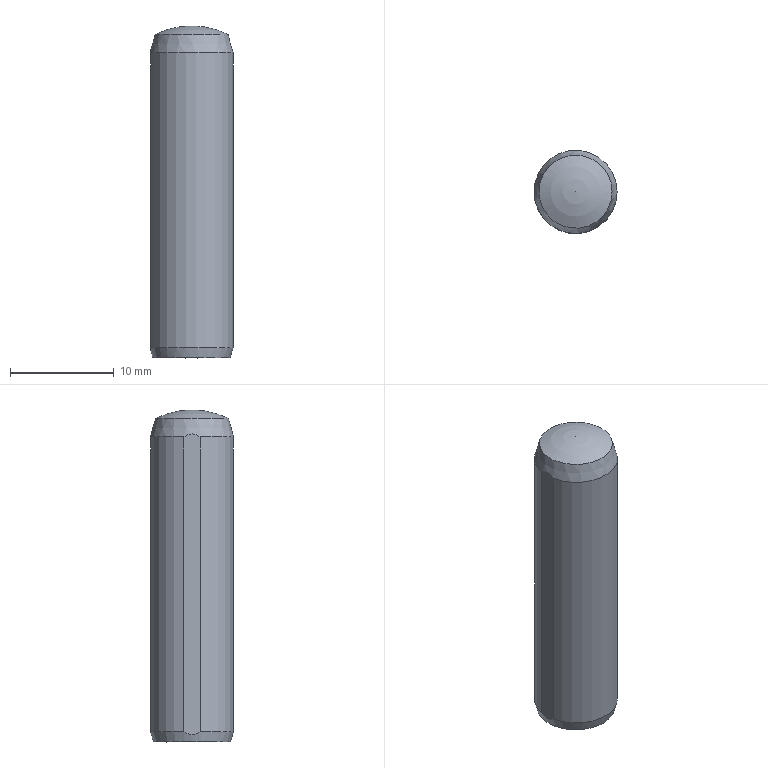Part | STEP file | 1_18 | 1 solid | 12 faces | box 7.92 x 8 x 32 mm | volume 1366 mm3 | cone 5 | cylinder 3 | plane 3 | sphere 1 | commonest cylinder face diameters 4.134 x2 8 x1
STEP:
#1=CARTESIAN_POINT('',(0.,0.,0.));
#2=DIRECTION('',(0.,0.,1.));
#3=DIRECTION('',(1.,0.,0.));
#4=AXIS2_PLACEMENT_3D('',#1,#2,#3);
#5=CARTESIAN_POINT('',(-3.92,-0.796,29.4));
#6=VERTEX_POINT('',#5);
#7=CARTESIAN_POINT('',(-3.92,0.796,29.4));
#8=VERTEX_POINT('',#7);
#9=CARTESIAN_POINT('',(0.,0.,29.4));
#10=DIRECTION('',(0.,0.,1.));
#11=DIRECTION('',(1.,0.,0.));
#12=AXIS2_PLACEMENT_3D('',#9,#10,#11);
#13=CIRCLE('',#12,4.);
#14=CARTESIAN_POINT('',(0.,0.,15.2));
#15=DIRECTION('',(0.,0.,1.));
#16=DIRECTION('',(0.,1.,0.));
#17=AXIS2_PLACEMENT_3D('',#14,#15,#16);
#18=CYLINDRICAL_SURFACE('',#17,4.);
#19=CARTESIAN_POINT('',(-1.571,14.2));
#20=DIRECTION('',(1.,0.));
#21=VECTOR('',#20,1.);
#22=LINE('',#19,#21);
#23=(GEOMETRIC_REPRESENTATION_CONTEXT(2)PARAMETRIC_REPRESENTATION_CONTEXT()REPRESENTATION_CONTEXT('',''));
#24=DEFINITIONAL_REPRESENTATION('',(#22),#23);
#25=PCURVE('',#18,#24);
#26=CARTESIAN_POINT('',(0.,0.,30.291));
#27=DIRECTION('',(0.,0.,-1.));
#28=DIRECTION('',(0.,-1.,0.));
#29=AXIS2_PLACEMENT_3D('',#26,#27,#28);
#30=CONICAL_SURFACE('',#29,3.761,0.2618);
#31=CARTESIAN_POINT('',(10.996,0.8914));
#32=DIRECTION('',(-1.,0.));
#33=VECTOR('',#32,1.);
#34=LINE('',#31,#33);
#35=(GEOMETRIC_REPRESENTATION_CONTEXT(2)PARAMETRIC_REPRESENTATION_CONTEXT()REPRESENTATION_CONTEXT('',''));
#36=DEFINITIONAL_REPRESENTATION('',(#34),#35);
#37=PCURVE('',#30,#36);
#38=SURFACE_CURVE('',#13,(#25,#37),.PCURVE_S1.);
#39=EDGE_CURVE('',#6,#8,#38,.T.);
#40=ORIENTED_EDGE('',*,*,#39,.F.);
#41=CARTESIAN_POINT('',(-3.92,-0.796,1.));
#42=VERTEX_POINT('',#41);
#43=CARTESIAN_POINT('',(-3.92,-0.796,1.));
#44=DIRECTION('',(0.,0.,1.));
#45=VECTOR('',#44,1.);
#46=LINE('',#43,#45);
#47=CARTESIAN_POINT('',(1.771,-14.2));
#48=DIRECTION('',(0.,1.));
#49=VECTOR('',#48,1.);
#50=LINE('',#47,#49);
#51=(GEOMETRIC_REPRESENTATION_CONTEXT(2)PARAMETRIC_REPRESENTATION_CONTEXT()REPRESENTATION_CONTEXT('',''));
#52=DEFINITIONAL_REPRESENTATION('',(#50),#51);
#53=PCURVE('',#18,#52);
#54=CARTESIAN_POINT('',(-3.92,0.,15.9));
#55=DIRECTION('',(-1.,0.,0.));
#56=DIRECTION('',(0.,0.,1.));
#57=AXIS2_PLACEMENT_3D('',#54,#55,#56);
#58=PLANE('',#57);
#59=CARTESIAN_POINT('',(-14.9,-0.796));
#60=DIRECTION('',(1.,0.));
#61=VECTOR('',#60,1.);
#62=LINE('',#59,#61);
#63=(GEOMETRIC_REPRESENTATION_CONTEXT(2)PARAMETRIC_REPRESENTATION_CONTEXT()REPRESENTATION_CONTEXT('',''));
#64=DEFINITIONAL_REPRESENTATION('',(#62),#63);
#65=PCURVE('',#58,#64);
#66=SURFACE_CURVE('',#46,(#53,#65),.PCURVE_S1.);
#67=EDGE_CURVE('',#42,#6,#66,.T.);
#68=ORIENTED_EDGE('',*,*,#67,.F.);
#69=CARTESIAN_POINT('',(-3.92,0.796,1.));
#70=VERTEX_POINT('',#69);
#71=CARTESIAN_POINT('',(0.,0.,1.));
#72=DIRECTION('',(0.,0.,1.));
#73=DIRECTION('',(1.,0.,0.));
#74=AXIS2_PLACEMENT_3D('',#71,#72,#73);
#75=CIRCLE('',#74,4.);
#76=CARTESIAN_POINT('',(-1.571,-14.2));
#77=DIRECTION('',(1.,0.));
#78=VECTOR('',#77,1.);
#79=LINE('',#76,#78);
#80=(GEOMETRIC_REPRESENTATION_CONTEXT(2)PARAMETRIC_REPRESENTATION_CONTEXT()REPRESENTATION_CONTEXT('',''));
#81=DEFINITIONAL_REPRESENTATION('',(#79),#80);
#82=PCURVE('',#18,#81);
#83=CARTESIAN_POINT('',(0.,0.,0.5));
#84=DIRECTION('',(0.,0.,1.));
#85=DIRECTION('',(0.,1.,0.));
#86=AXIS2_PLACEMENT_3D('',#83,#84,#85);
#87=CONICAL_SURFACE('',#86,3.866,0.2618);
#88=CARTESIAN_POINT('',(-1.571,0.5));
#89=DIRECTION('',(1.,0.));
#90=VECTOR('',#89,1.);
#91=LINE('',#88,#90);
#92=(GEOMETRIC_REPRESENTATION_CONTEXT(2)PARAMETRIC_REPRESENTATION_CONTEXT()REPRESENTATION_CONTEXT('',''));
#93=DEFINITIONAL_REPRESENTATION('',(#91),#92);
#94=PCURVE('',#87,#93);
#95=SURFACE_CURVE('',#75,(#82,#94),.PCURVE_S1.);
#96=EDGE_CURVE('',#42,#70,#95,.T.);
#97=ORIENTED_EDGE('',*,*,#96,.T.);
#98=CARTESIAN_POINT('',(-3.92,0.796,1.));
#99=DIRECTION('',(0.,0.,1.));
#100=VECTOR('',#99,1.);
#101=LINE('',#98,#100);
#102=CARTESIAN_POINT('',(7.654,-14.2));
#103=DIRECTION('',(0.,1.));
#104=VECTOR('',#103,1.);
#105=LINE('',#102,#104);
#106=(GEOMETRIC_REPRESENTATION_CONTEXT(2)PARAMETRIC_REPRESENTATION_CONTEXT()REPRESENTATION_CONTEXT('',''));
#107=DEFINITIONAL_REPRESENTATION('',(#105),#106);
#108=PCURVE('',#18,#107);
#109=CARTESIAN_POINT('',(-14.9,0.796));
#110=DIRECTION('',(1.,0.));
#111=VECTOR('',#110,1.);
#112=LINE('',#109,#111);
#113=(GEOMETRIC_REPRESENTATION_CONTEXT(2)PARAMETRIC_REPRESENTATION_CONTEXT()REPRESENTATION_CONTEXT('',''));
#114=DEFINITIONAL_REPRESENTATION('',(#112),#113);
#115=PCURVE('',#58,#114);
#116=SURFACE_CURVE('',#101,(#108,#115),.PCURVE_S1.);
#117=EDGE_CURVE('',#70,#8,#116,.T.);
#118=ORIENTED_EDGE('',*,*,#117,.T.);
#119=EDGE_LOOP('',(#40,#68,#97,#118));
#120=FACE_BOUND('',#119,.T.);
#121=ADVANCED_FACE('',(#120),#18,.T.);
#122=CARTESIAN_POINT('',(-3.522,0.,31.183));
#123=VERTEX_POINT('',#122);
#124=CARTESIAN_POINT('',(3.522,0.,31.183));
#125=VERTEX_POINT('',#124);
#126=CARTESIAN_POINT('',(0.,0.,31.183));
#127=DIRECTION('',(0.,0.,-1.));
#128=DIRECTION('',(1.,0.,0.));
#129=AXIS2_PLACEMENT_3D('',#126,#127,#128);
#130=CIRCLE('',#129,3.522);
#131=CARTESIAN_POINT('',(-1.571,-0.8914));
#132=DIRECTION('',(1.,0.));
#133=VECTOR('',#132,1.);
#134=LINE('',#131,#133);
#135=(GEOMETRIC_REPRESENTATION_CONTEXT(2)PARAMETRIC_REPRESENTATION_CONTEXT()REPRESENTATION_CONTEXT('',''));
#136=DEFINITIONAL_REPRESENTATION('',(#134),#135);
#137=PCURVE('',#30,#136);
#138=CARTESIAN_POINT('',(0.,0.,24.));
#139=DIRECTION('',(0.,0.,1.));
#140=DIRECTION('',(1.,0.,0.));
#141=AXIS2_PLACEMENT_3D('',#138,#139,#140);
#142=SPHERICAL_SURFACE('',#141,8.);
#143=CARTESIAN_POINT('',(3.142,1.115));
#144=CARTESIAN_POINT('',(3.049,1.115));
#145=CARTESIAN_POINT('',(2.865,1.115));
#146=CARTESIAN_POINT('',(2.589,1.115));
#147=CARTESIAN_POINT('',(2.312,1.115));
#148=CARTESIAN_POINT('',(2.036,1.115));
#149=CARTESIAN_POINT('',(1.759,1.115));
#150=CARTESIAN_POINT('',(1.483,1.115));
#151=CARTESIAN_POINT('',(1.206,1.115));
#152=CARTESIAN_POINT('',(0.9296,1.115));
#153=CARTESIAN_POINT('',(0.6532,1.115));
#154=CARTESIAN_POINT('',(0.3767,1.115));
#155=CARTESIAN_POINT('',(0.1002,1.115));
#156=CARTESIAN_POINT('',(-0.1763,1.115));
#157=CARTESIAN_POINT('',(-0.4528,1.115));
#158=CARTESIAN_POINT('',(-0.7293,1.115));
#159=CARTESIAN_POINT('',(-1.006,1.115));
#160=CARTESIAN_POINT('',(-1.282,1.115));
#161=CARTESIAN_POINT('',(-1.559,1.115));
#162=CARTESIAN_POINT('',(-1.835,1.115));
#163=CARTESIAN_POINT('',(-2.112,1.115));
#164=CARTESIAN_POINT('',(-2.388,1.115));
#165=CARTESIAN_POINT('',(-2.665,1.115));
#166=CARTESIAN_POINT('',(-2.849,1.115));
#167=CARTESIAN_POINT('',(-2.941,1.115));
#168=B_SPLINE_CURVE_WITH_KNOTS('',3,(#143,#144,#145,#146,#147,#148,#149,#150,#151,#152,#153,#154,#155,#156,#157,#158,#159,#160,#161,#162,#163,#164,#165,#166,#167),.UNSPECIFIED.,.F.,.F.,(4,1,1,1,1,1,1,1,1,1,1,1,1,1,1,1,1,1,1,1,1,1,4),(3.142,3.418,3.695,3.971,4.248,4.524,4.801,5.077,5.354,5.63,5.907,6.183,6.46,6.736,7.012,7.289,7.565,7.842,8.118,8.395,8.671,8.948,9.224),.QUASI_UNIFORM_KNOTS.);
#169=(GEOMETRIC_REPRESENTATION_CONTEXT(2)PARAMETRIC_REPRESENTATION_CONTEXT()REPRESENTATION_CONTEXT('',''));
#170=DEFINITIONAL_REPRESENTATION('',(#168),#169);
#171=PCURVE('',#142,#170);
#172=SURFACE_CURVE('',#130,(#137,#171),.PCURVE_S1.);
#173=EDGE_CURVE('',#123,#125,#172,.T.);
#174=ORIENTED_EDGE('',*,*,#173,.T.);
#175=CARTESIAN_POINT('',(-3.452,-0.7009,31.183));
#176=VERTEX_POINT('',#175);
#177=CARTESIAN_POINT('',(0.,0.,31.183));
#178=DIRECTION('',(0.,0.,-1.));
#179=DIRECTION('',(1.,0.,0.));
#180=AXIS2_PLACEMENT_3D('',#177,#178,#179);
#181=CIRCLE('',#180,3.522);
#182=CARTESIAN_POINT('',(-1.571,-0.8914));
#183=DIRECTION('',(1.,0.));
#184=VECTOR('',#183,1.);
#185=LINE('',#182,#184);
#186=(GEOMETRIC_REPRESENTATION_CONTEXT(2)PARAMETRIC_REPRESENTATION_CONTEXT()REPRESENTATION_CONTEXT('',''));
#187=DEFINITIONAL_REPRESENTATION('',(#185),#186);
#188=PCURVE('',#30,#187);
#189=CARTESIAN_POINT('',(9.425,1.115));
#190=CARTESIAN_POINT('',(9.333,1.115));
#191=CARTESIAN_POINT('',(9.148,1.115));
#192=CARTESIAN_POINT('',(8.872,1.115));
#193=CARTESIAN_POINT('',(8.595,1.115));
#194=CARTESIAN_POINT('',(8.319,1.115));
#195=CARTESIAN_POINT('',(8.042,1.115));
#196=CARTESIAN_POINT('',(7.766,1.115));
#197=CARTESIAN_POINT('',(7.489,1.115));
#198=CARTESIAN_POINT('',(7.213,1.115));
#199=CARTESIAN_POINT('',(6.936,1.115));
#200=CARTESIAN_POINT('',(6.66,1.115));
#201=CARTESIAN_POINT('',(6.383,1.115));
#202=CARTESIAN_POINT('',(6.107,1.115));
#203=CARTESIAN_POINT('',(5.83,1.115));
#204=CARTESIAN_POINT('',(5.554,1.115));
#205=CARTESIAN_POINT('',(5.277,1.115));
#206=CARTESIAN_POINT('',(5.001,1.115));
#207=CARTESIAN_POINT('',(4.724,1.115));
#208=CARTESIAN_POINT('',(4.448,1.115));
#209=CARTESIAN_POINT('',(4.171,1.115));
#210=CARTESIAN_POINT('',(3.895,1.115));
#211=CARTESIAN_POINT('',(3.618,1.115));
#212=CARTESIAN_POINT('',(3.434,1.115));
#213=CARTESIAN_POINT('',(3.342,1.115));
#214=B_SPLINE_CURVE_WITH_KNOTS('',3,(#189,#190,#191,#192,#193,#194,#195,#196,#197,#198,#199,#200,#201,#202,#203,#204,#205,#206,#207,#208,#209,#210,#211,#212,#213),.UNSPECIFIED.,.F.,.F.,(4,1,1,1,1,1,1,1,1,1,1,1,1,1,1,1,1,1,1,1,1,1,4),(3.142,3.418,3.695,3.971,4.248,4.524,4.801,5.077,5.354,5.63,5.907,6.183,6.46,6.736,7.012,7.289,7.565,7.842,8.118,8.395,8.671,8.948,9.224),.QUASI_UNIFORM_KNOTS.);
#215=(GEOMETRIC_REPRESENTATION_CONTEXT(2)PARAMETRIC_REPRESENTATION_CONTEXT()REPRESENTATION_CONTEXT('',''));
#216=DEFINITIONAL_REPRESENTATION('',(#214),#215);
#217=PCURVE('',#142,#216);
#218=SURFACE_CURVE('',#181,(#188,#217),.PCURVE_S1.);
#219=EDGE_CURVE('',#125,#176,#218,.T.);
#220=ORIENTED_EDGE('',*,*,#219,.T.);
#221=CARTESIAN_POINT('',(-3.452,-0.7009,31.183));
#222=CARTESIAN_POINT('',(-3.92,-0.796,29.4));
#223=B_SPLINE_CURVE_WITH_KNOTS('',1,(#221,#222),.UNSPECIFIED.,.F.,.F.,(2,2),(-0.9229,0.9229),.PIECEWISE_BEZIER_KNOTS.);
#224=CARTESIAN_POINT('',(7.654,0.));
#225=DIRECTION('',(0.,1.));
#226=VECTOR('',#225,1.);
#227=LINE('',#224,#226);
#228=(GEOMETRIC_REPRESENTATION_CONTEXT(2)PARAMETRIC_REPRESENTATION_CONTEXT()REPRESENTATION_CONTEXT('',''));
#229=DEFINITIONAL_REPRESENTATION('',(#227),#228);
#230=PCURVE('',#30,#229);
#231=CARTESIAN_POINT('',(1.37,0.));
#232=DIRECTION('',(0.,1.));
#233=VECTOR('',#232,1.);
#234=LINE('',#231,#233);
#235=(GEOMETRIC_REPRESENTATION_CONTEXT(2)PARAMETRIC_REPRESENTATION_CONTEXT()REPRESENTATION_CONTEXT('',''));
#236=DEFINITIONAL_REPRESENTATION('',(#234),#235);
#237=PCURVE('',#30,#236);
#238=SEAM_CURVE('',#223,(#230,#237),.PCURVE_S1.);
#239=EDGE_CURVE('',#176,#6,#238,.T.);
#240=ORIENTED_EDGE('',*,*,#239,.T.);
#241=ORIENTED_EDGE('',*,*,#39,.T.);
#242=CARTESIAN_POINT('',(-3.92,0.796,29.4));
#243=CARTESIAN_POINT('',(-3.92,0.3871,29.704));
#244=CARTESIAN_POINT('',(-3.92,0.,29.791));
#245=CARTESIAN_POINT('',(-3.92,-0.3871,29.704));
#246=CARTESIAN_POINT('',(-3.92,-0.796,29.4));
#247=B_SPLINE_CURVE_WITH_KNOTS('',4,(#242,#243,#244,#245,#246),.UNSPECIFIED.,.F.,.F.,(5,5),(0.,40.137),.PIECEWISE_BEZIER_KNOTS.);
#248=CARTESIAN_POINT('',(1.771,0.8914));
#249=CARTESIAN_POINT('',(1.765,0.873));
#250=CARTESIAN_POINT('',(1.753,0.838));
#251=CARTESIAN_POINT('',(1.735,0.7907));
#252=CARTESIAN_POINT('',(1.716,0.7487));
#253=CARTESIAN_POINT('',(1.698,0.7117));
#254=CARTESIAN_POINT('',(1.68,0.6798));
#255=CARTESIAN_POINT('',(1.662,0.6529));
#256=CARTESIAN_POINT('',(1.644,0.6309));
#257=CARTESIAN_POINT('',(1.625,0.6139));
#258=CARTESIAN_POINT('',(1.607,0.6018));
#259=CARTESIAN_POINT('',(1.589,0.5945));
#260=CARTESIAN_POINT('',(1.571,0.5921));
#261=CARTESIAN_POINT('',(1.553,0.5945));
#262=CARTESIAN_POINT('',(1.534,0.6018));
#263=CARTESIAN_POINT('',(1.516,0.6139));
#264=CARTESIAN_POINT('',(1.498,0.6309));
#265=CARTESIAN_POINT('',(1.48,0.6529));
#266=CARTESIAN_POINT('',(1.462,0.6798));
#267=CARTESIAN_POINT('',(1.443,0.7117));
#268=CARTESIAN_POINT('',(1.425,0.7487));
#269=CARTESIAN_POINT('',(1.407,0.7907));
#270=CARTESIAN_POINT('',(1.389,0.838));
#271=CARTESIAN_POINT('',(1.377,0.873));
#272=CARTESIAN_POINT('',(1.37,0.8914));
#273=B_SPLINE_CURVE_WITH_KNOTS('',3,(#248,#249,#250,#251,#252,#253,#254,#255,#256,#257,#258,#259,#260,#261,#262,#263,#264,#265,#266,#267,#268,#269,#270,#271,#272),.UNSPECIFIED.,.F.,.F.,(4,1,1,1,1,1,1,1,1,1,1,1,1,1,1,1,1,1,1,1,1,1,4),(0.,1.824,3.649,5.473,7.298,9.122,10.946,12.771,14.595,16.419,18.244,20.068,21.893,23.717,25.541,27.366,29.19,31.015,32.839,34.663,36.488,38.312,40.137),.QUASI_UNIFORM_KNOTS.);
#274=(GEOMETRIC_REPRESENTATION_CONTEXT(2)PARAMETRIC_REPRESENTATION_CONTEXT()REPRESENTATION_CONTEXT('',''));
#275=DEFINITIONAL_REPRESENTATION('',(#273),#274);
#276=PCURVE('',#30,#275);
#277=CARTESIAN_POINT('',(13.5,0.796));
#278=CARTESIAN_POINT('',(13.804,0.3871));
#279=CARTESIAN_POINT('',(13.891,0.));
#280=CARTESIAN_POINT('',(13.804,-0.3871));
#281=CARTESIAN_POINT('',(13.5,-0.796));
#282=B_SPLINE_CURVE_WITH_KNOTS('',4,(#277,#278,#279,#280,#281),.UNSPECIFIED.,.F.,.F.,(5,5),(0.,40.137),.PIECEWISE_BEZIER_KNOTS.);
#283=(GEOMETRIC_REPRESENTATION_CONTEXT(2)PARAMETRIC_REPRESENTATION_CONTEXT()REPRESENTATION_CONTEXT('',''));
#284=DEFINITIONAL_REPRESENTATION('',(#282),#283);
#285=PCURVE('',#58,#284);
#286=SURFACE_CURVE('',#247,(#276,#285),.PCURVE_S1.);
#287=EDGE_CURVE('',#8,#6,#286,.T.);
#288=ORIENTED_EDGE('',*,*,#287,.T.);
#289=ORIENTED_EDGE('',*,*,#239,.F.);
#290=CARTESIAN_POINT('',(0.,0.,31.183));
#291=DIRECTION('',(0.,0.,-1.));
#292=DIRECTION('',(1.,0.,0.));
#293=AXIS2_PLACEMENT_3D('',#290,#291,#292);
#294=CIRCLE('',#293,3.522);
#295=CARTESIAN_POINT('',(-1.571,-0.8914));
#296=DIRECTION('',(1.,0.));
#297=VECTOR('',#296,1.);
#298=LINE('',#295,#297);
#299=(GEOMETRIC_REPRESENTATION_CONTEXT(2)PARAMETRIC_REPRESENTATION_CONTEXT()REPRESENTATION_CONTEXT('',''));
#300=DEFINITIONAL_REPRESENTATION('',(#298),#299);
#301=PCURVE('',#30,#300);
#302=CARTESIAN_POINT('',(6.283,1.115));
#303=DIRECTION('',(-1.,0.));
#304=VECTOR('',#303,1.);
#305=LINE('',#302,#304);
#306=(GEOMETRIC_REPRESENTATION_CONTEXT(2)PARAMETRIC_REPRESENTATION_CONTEXT()REPRESENTATION_CONTEXT('',''));
#307=DEFINITIONAL_REPRESENTATION('',(#305),#306);
#308=PCURVE('',#142,#307);
#309=SURFACE_CURVE('',#294,(#301,#308),.PCURVE_S1.);
#310=EDGE_CURVE('',#176,#123,#309,.T.);
#311=ORIENTED_EDGE('',*,*,#310,.T.);
#312=EDGE_LOOP('',(#174,#220,#240,#241,#288,#289,#311));
#313=FACE_BOUND('',#312,.T.);
#314=ADVANCED_FACE('',(#313),#30,.T.);
#315=ORIENTED_EDGE('',*,*,#287,.F.);
#316=ORIENTED_EDGE('',*,*,#117,.F.);
#317=CARTESIAN_POINT('',(-3.92,-0.796,1.));
#318=CARTESIAN_POINT('',(-3.92,-0.6482,0.8903));
#319=CARTESIAN_POINT('',(-3.92,-0.4955,0.8013));
#320=CARTESIAN_POINT('',(-3.92,-0.3382,0.7376));
#321=CARTESIAN_POINT('',(-3.92,-0.019,0.6712));
#322=CARTESIAN_POINT('',(-3.92,0.3008,0.7264));
#323=CARTESIAN_POINT('',(-3.92,0.4576,0.7842));
#324=CARTESIAN_POINT('',(-3.92,0.6181,0.872));
#325=CARTESIAN_POINT('',(-3.92,0.7732,0.9832));
#326=CARTESIAN_POINT('',(-3.92,0.7808,0.9888));
#327=CARTESIAN_POINT('',(-3.92,0.7884,0.9944));
#328=CARTESIAN_POINT('',(-3.92,0.796,1.));
#329=B_SPLINE_CURVE_WITH_KNOTS('',5,(#317,#318,#319,#320,#321,#322,#323,#324,#325,#326,#327,#328),.UNSPECIFIED.,.F.,.F.,(6,3,3,6),(0.,1.289,2.568,2.634),.UNSPECIFIED.);
#330=CARTESIAN_POINT('',(-14.9,-0.796));
#331=CARTESIAN_POINT('',(-15.01,-0.6482));
#332=CARTESIAN_POINT('',(-15.099,-0.4955));
#333=CARTESIAN_POINT('',(-15.162,-0.3382));
#334=CARTESIAN_POINT('',(-15.229,-0.019));
#335=CARTESIAN_POINT('',(-15.174,0.3008));
#336=CARTESIAN_POINT('',(-15.116,0.4576));
#337=CARTESIAN_POINT('',(-15.028,0.6181));
#338=CARTESIAN_POINT('',(-14.917,0.7732));
#339=CARTESIAN_POINT('',(-14.911,0.7808));
#340=CARTESIAN_POINT('',(-14.906,0.7884));
#341=CARTESIAN_POINT('',(-14.9,0.796));
#342=B_SPLINE_CURVE_WITH_KNOTS('',5,(#330,#331,#332,#333,#334,#335,#336,#337,#338,#339,#340,#341),.UNSPECIFIED.,.F.,.F.,(6,3,3,6),(0.,1.289,2.568,2.634),.UNSPECIFIED.);
#343=(GEOMETRIC_REPRESENTATION_CONTEXT(2)PARAMETRIC_REPRESENTATION_CONTEXT()REPRESENTATION_CONTEXT('',''));
#344=DEFINITIONAL_REPRESENTATION('',(#342),#343);
#345=PCURVE('',#58,#344);
#346=CARTESIAN_POINT('',(1.771,0.5));
#347=CARTESIAN_POINT('',(1.766,0.483));
#348=CARTESIAN_POINT('',(1.754,0.4502));
#349=CARTESIAN_POINT('',(1.737,0.4048));
#350=CARTESIAN_POINT('',(1.719,0.3635));
#351=CARTESIAN_POINT('',(1.701,0.3263));
#352=CARTESIAN_POINT('',(1.683,0.2937));
#353=CARTESIAN_POINT('',(1.665,0.2656));
#354=CARTESIAN_POINT('',(1.646,0.2424));
#355=CARTESIAN_POINT('',(1.628,0.2242));
#356=CARTESIAN_POINT('',(1.609,0.2111));
#357=CARTESIAN_POINT('',(1.59,0.2032));
#358=CARTESIAN_POINT('',(1.571,0.2006));
#359=CARTESIAN_POINT('',(1.552,0.2032));
#360=CARTESIAN_POINT('',(1.533,0.2111));
#361=CARTESIAN_POINT('',(1.514,0.2242));
#362=CARTESIAN_POINT('',(1.495,0.2424));
#363=CARTESIAN_POINT('',(1.477,0.2656));
#364=CARTESIAN_POINT('',(1.458,0.2937));
#365=CARTESIAN_POINT('',(1.44,0.3263));
#366=CARTESIAN_POINT('',(1.422,0.3635));
#367=CARTESIAN_POINT('',(1.405,0.4048));
#368=CARTESIAN_POINT('',(1.387,0.4502));
#369=CARTESIAN_POINT('',(1.376,0.483));
#370=CARTESIAN_POINT('',(1.37,0.5));
#371=B_SPLINE_CURVE_WITH_KNOTS('',3,(#346,#347,#348,#349,#350,#351,#352,#353,#354,#355,#356,#357,#358,#359,#360,#361,#362,#363,#364,#365,#366,#367,#368,#369,#370),.UNSPECIFIED.,.F.,.F.,(4,1,1,1,1,1,1,1,1,1,1,1,1,1,1,1,1,1,1,1,1,1,4),(0.,0.1197,0.2395,0.3592,0.4789,0.5987,0.7184,0.8381,0.9579,1.078,1.197,1.317,1.437,1.557,1.676,1.796,1.916,2.035,2.155,2.275,2.395,2.514,2.634),.QUASI_UNIFORM_KNOTS.);
#372=(GEOMETRIC_REPRESENTATION_CONTEXT(2)PARAMETRIC_REPRESENTATION_CONTEXT()REPRESENTATION_CONTEXT('',''));
#373=DEFINITIONAL_REPRESENTATION('',(#371),#372);
#374=PCURVE('',#87,#373);
#375=SURFACE_CURVE('',#329,(#345,#374),.PCURVE_S1.);
#376=EDGE_CURVE('',#42,#70,#375,.T.);
#377=ORIENTED_EDGE('',*,*,#376,.F.);
#378=ORIENTED_EDGE('',*,*,#67,.T.);
#379=EDGE_LOOP('',(#315,#316,#377,#378));
#380=FACE_BOUND('',#379,.T.);
#381=ADVANCED_FACE('',(#380),#58,.T.);
#382=ORIENTED_EDGE('',*,*,#96,.F.);
#383=ORIENTED_EDGE('',*,*,#376,.T.);
#384=CARTESIAN_POINT('',(-3.657,0.7427,0.));
#385=VERTEX_POINT('',#384);
#386=CARTESIAN_POINT('',(-3.657,0.7427,0.));
#387=CARTESIAN_POINT('',(-3.92,0.796,1.));
#388=B_SPLINE_CURVE_WITH_KNOTS('',1,(#386,#387),.UNSPECIFIED.,.F.,.F.,(2,2),(-0.5176,0.5176),.PIECEWISE_BEZIER_KNOTS.);
#389=CARTESIAN_POINT('',(1.37,0.));
#390=DIRECTION('',(0.,1.));
#391=VECTOR('',#390,1.);
#392=LINE('',#389,#391);
#393=(GEOMETRIC_REPRESENTATION_CONTEXT(2)PARAMETRIC_REPRESENTATION_CONTEXT()REPRESENTATION_CONTEXT('',''));
#394=DEFINITIONAL_REPRESENTATION('',(#392),#393);
#395=PCURVE('',#87,#394);
#396=CARTESIAN_POINT('',(7.654,0.));
#397=DIRECTION('',(0.,1.));
#398=VECTOR('',#397,1.);
#399=LINE('',#396,#398);
#400=(GEOMETRIC_REPRESENTATION_CONTEXT(2)PARAMETRIC_REPRESENTATION_CONTEXT()REPRESENTATION_CONTEXT('',''));
#401=DEFINITIONAL_REPRESENTATION('',(#399),#400);
#402=PCURVE('',#87,#401);
#403=SEAM_CURVE('',#388,(#395,#402),.PCURVE_S1.);
#404=EDGE_CURVE('',#385,#70,#403,.T.);
#405=ORIENTED_EDGE('',*,*,#404,.F.);
#406=CARTESIAN_POINT('',(0.,-3.732,0.));
#407=VERTEX_POINT('',#406);
#408=CARTESIAN_POINT('',(0.,0.,0.));
#409=DIRECTION('',(0.,0.,1.));
#410=DIRECTION('',(1.,0.,0.));
#411=AXIS2_PLACEMENT_3D('',#408,#409,#410);
#412=CIRCLE('',#411,3.732);
#413=CARTESIAN_POINT('',(-1.571,-0.5));
#414=DIRECTION('',(1.,0.));
#415=VECTOR('',#414,1.);
#416=LINE('',#413,#415);
#417=(GEOMETRIC_REPRESENTATION_CONTEXT(2)PARAMETRIC_REPRESENTATION_CONTEXT()REPRESENTATION_CONTEXT('',''));
#418=DEFINITIONAL_REPRESENTATION('',(#416),#417);
#419=PCURVE('',#87,#418);
#420=CARTESIAN_POINT('',(0.,1.866,0.));
#421=DIRECTION('',(0.,0.,-1.));
#422=DIRECTION('',(-1.,0.,0.));
#423=AXIS2_PLACEMENT_3D('',#420,#421,#422);
#424=PLANE('',#423);
#425=CARTESIAN_POINT('',(-3.732,-1.866));
#426=CARTESIAN_POINT('',(-3.732,4.598));
#427=CARTESIAN_POINT('',(1.866,1.366));
#428=CARTESIAN_POINT('',(7.464,-1.866));
#429=CARTESIAN_POINT('',(1.866,-5.098));
#430=CARTESIAN_POINT('',(-3.732,-8.33));
#431=CARTESIAN_POINT('',(-3.732,-1.866));
#432=(BOUNDED_CURVE()B_SPLINE_CURVE(2,(#425,#426,#427,#428,#429,#430,#431),.UNSPECIFIED.,.T.,.F.)B_SPLINE_CURVE_WITH_KNOTS((1,2,2,2,2,1),(-2.094,0.,2.094,4.189,6.283,8.378),.UNSPECIFIED.)CURVE()GEOMETRIC_REPRESENTATION_ITEM()RATIONAL_B_SPLINE_CURVE((1.,0.5,1.,0.5,1.,0.5,1.))REPRESENTATION_ITEM(''));
#433=(GEOMETRIC_REPRESENTATION_CONTEXT(2)PARAMETRIC_REPRESENTATION_CONTEXT()REPRESENTATION_CONTEXT('',''));
#434=DEFINITIONAL_REPRESENTATION('',(#432),#433);
#435=PCURVE('',#424,#434);
#436=SURFACE_CURVE('',#412,(#419,#435),.PCURVE_S1.);
#437=EDGE_CURVE('',#385,#407,#436,.T.);
#438=ORIENTED_EDGE('',*,*,#437,.T.);
#439=CARTESIAN_POINT('',(0.,0.,0.));
#440=DIRECTION('',(0.,0.,1.));
#441=DIRECTION('',(1.,0.,0.));
#442=AXIS2_PLACEMENT_3D('',#439,#440,#441);
#443=CIRCLE('',#442,3.732);
#444=CARTESIAN_POINT('',(-1.571,-0.5));
#445=DIRECTION('',(1.,0.));
#446=VECTOR('',#445,1.);
#447=LINE('',#444,#446);
#448=(GEOMETRIC_REPRESENTATION_CONTEXT(2)PARAMETRIC_REPRESENTATION_CONTEXT()REPRESENTATION_CONTEXT('',''));
#449=DEFINITIONAL_REPRESENTATION('',(#447),#448);
#450=PCURVE('',#87,#449);
#451=CARTESIAN_POINT('',(-3.732,-1.866));
#452=CARTESIAN_POINT('',(-3.732,4.598));
#453=CARTESIAN_POINT('',(1.866,1.366));
#454=CARTESIAN_POINT('',(7.464,-1.866));
#455=CARTESIAN_POINT('',(1.866,-5.098));
#456=CARTESIAN_POINT('',(-3.732,-8.33));
#457=CARTESIAN_POINT('',(-3.732,-1.866));
#458=(BOUNDED_CURVE()B_SPLINE_CURVE(2,(#451,#452,#453,#454,#455,#456,#457),.UNSPECIFIED.,.T.,.F.)B_SPLINE_CURVE_WITH_KNOTS((1,2,2,2,2,1),(-2.094,0.,2.094,4.189,6.283,8.378),.UNSPECIFIED.)CURVE()GEOMETRIC_REPRESENTATION_ITEM()RATIONAL_B_SPLINE_CURVE((1.,0.5,1.,0.5,1.,0.5,1.))REPRESENTATION_ITEM(''));
#459=(GEOMETRIC_REPRESENTATION_CONTEXT(2)PARAMETRIC_REPRESENTATION_CONTEXT()REPRESENTATION_CONTEXT('',''));
#460=DEFINITIONAL_REPRESENTATION('',(#458),#459);
#461=PCURVE('',#424,#460);
#462=SURFACE_CURVE('',#443,(#450,#461),.PCURVE_S1.);
#463=EDGE_CURVE('',#407,#385,#462,.T.);
#464=ORIENTED_EDGE('',*,*,#463,.T.);
#465=ORIENTED_EDGE('',*,*,#404,.T.);
#466=EDGE_LOOP('',(#382,#383,#405,#438,#464,#465));
#467=FACE_BOUND('',#466,.T.);
#468=ADVANCED_FACE('',(#467),#87,.T.);
#469=ORIENTED_EDGE('',*,*,#219,.F.);
#470=CARTESIAN_POINT('',(0.,0.,32.));
#471=VERTEX_POINT('',#470);
#472=CARTESIAN_POINT('',(3.522,0.,31.183));
#473=CARTESIAN_POINT('',(2.867,0.,31.504));
#474=CARTESIAN_POINT('',(2.176,0.,31.751));
#475=CARTESIAN_POINT('',(1.459,0.,31.917));
#476=CARTESIAN_POINT('',(0.7295,0.,32.));
#477=CARTESIAN_POINT('',(0.,0.,32.));
#478=B_SPLINE_CURVE_WITH_KNOTS('',5,(#472,#473,#474,#475,#476,#477),.UNSPECIFIED.,.F.,.F.,(6,6),(1.115,1.571),.PIECEWISE_BEZIER_KNOTS.);
#479=CARTESIAN_POINT('',(6.283,0.));
#480=DIRECTION('',(0.,1.));
#481=VECTOR('',#480,1.);
#482=LINE('',#479,#481);
#483=(GEOMETRIC_REPRESENTATION_CONTEXT(2)PARAMETRIC_REPRESENTATION_CONTEXT()REPRESENTATION_CONTEXT('',''));
#484=DEFINITIONAL_REPRESENTATION('',(#482),#483);
#485=PCURVE('',#142,#484);
#486=CARTESIAN_POINT('',(0.,0.));
#487=DIRECTION('',(0.,1.));
#488=VECTOR('',#487,1.);
#489=LINE('',#486,#488);
#490=(GEOMETRIC_REPRESENTATION_CONTEXT(2)PARAMETRIC_REPRESENTATION_CONTEXT()REPRESENTATION_CONTEXT('',''));
#491=DEFINITIONAL_REPRESENTATION('',(#489),#490);
#492=PCURVE('',#142,#491);
#493=SEAM_CURVE('',#478,(#485,#492),.PCURVE_S1.);
#494=EDGE_CURVE('',#125,#471,#493,.T.);
#495=ORIENTED_EDGE('',*,*,#494,.T.);
#496=ORIENTED_EDGE('',*,*,#494,.F.);
#497=ORIENTED_EDGE('',*,*,#173,.F.);
#498=ORIENTED_EDGE('',*,*,#310,.F.);
#499=EDGE_LOOP('',(#469,#495,#496,#497,#498));
#500=FACE_BOUND('',#499,.T.);
#501=ADVANCED_FACE('',(#500),#142,.T.);
#502=ORIENTED_EDGE('',*,*,#463,.F.);
#503=ORIENTED_EDGE('',*,*,#437,.F.);
#504=EDGE_LOOP('',(#502,#503));
#505=FACE_BOUND('',#504,.T.);
#506=CARTESIAN_POINT('',(0.,2.5,0.));
#507=VERTEX_POINT('',#506);
#508=CARTESIAN_POINT('',(0.,0.,0.));
#509=DIRECTION('',(0.,0.,1.));
#510=DIRECTION('',(0.,1.,0.));
#511=AXIS2_PLACEMENT_3D('',#508,#509,#510);
#512=CIRCLE('',#511,2.5);
#513=CARTESIAN_POINT('',(0.,0.634));
#514=CARTESIAN_POINT('',(4.33,0.634));
#515=CARTESIAN_POINT('',(2.165,-3.116));
#516=CARTESIAN_POINT('',(0.,-6.866));
#517=CARTESIAN_POINT('',(-2.165,-3.116));
#518=CARTESIAN_POINT('',(-4.33,0.634));
#519=CARTESIAN_POINT('',(0.,0.634));
#520=(BOUNDED_CURVE()B_SPLINE_CURVE(2,(#513,#514,#515,#516,#517,#518,#519),.UNSPECIFIED.,.T.,.F.)B_SPLINE_CURVE_WITH_KNOTS((1,2,2,2,2,1),(-2.094,0.,2.094,4.189,6.283,8.378),.UNSPECIFIED.)CURVE()GEOMETRIC_REPRESENTATION_ITEM()RATIONAL_B_SPLINE_CURVE((1.,0.5,1.,0.5,1.,0.5,1.))REPRESENTATION_ITEM(''));
#521=(GEOMETRIC_REPRESENTATION_CONTEXT(2)PARAMETRIC_REPRESENTATION_CONTEXT()REPRESENTATION_CONTEXT('',''));
#522=DEFINITIONAL_REPRESENTATION('',(#520),#521);
#523=PCURVE('',#424,#522);
#524=CARTESIAN_POINT('',(0.,0.,0.2165));
#525=DIRECTION('',(0.,0.,-1.));
#526=DIRECTION('',(0.,1.,0.));
#527=AXIS2_PLACEMENT_3D('',#524,#525,#526);
#528=CONICAL_SURFACE('',#527,2.284,0.7854);
#529=CARTESIAN_POINT('',(6.283,0.2165));
#530=DIRECTION('',(-1.,0.));
#531=VECTOR('',#530,1.);
#532=LINE('',#529,#531);
#533=(GEOMETRIC_REPRESENTATION_CONTEXT(2)PARAMETRIC_REPRESENTATION_CONTEXT()REPRESENTATION_CONTEXT('',''));
#534=DEFINITIONAL_REPRESENTATION('',(#532),#533);
#535=PCURVE('',#528,#534);
#536=SURFACE_CURVE('',#512,(#523,#535),.PCURVE_S1.);
#537=EDGE_CURVE('',#507,#507,#536,.T.);
#538=ORIENTED_EDGE('',*,*,#537,.T.);
#539=EDGE_LOOP('',(#538));
#540=FACE_BOUND('',#539,.T.);
#541=ADVANCED_FACE('',(#505,#540),#424,.T.);
#542=ORIENTED_EDGE('',*,*,#537,.T.);
#543=CARTESIAN_POINT('',(0.,2.067,0.433));
#544=VERTEX_POINT('',#543);
#545=CARTESIAN_POINT('',(0.,2.067,0.433));
#546=CARTESIAN_POINT('',(0.,2.5,-0.000000001));
#547=B_SPLINE_CURVE_WITH_KNOTS('',1,(#545,#546),.UNSPECIFIED.,.F.,.F.,(2,2),(-0.3062,0.3062),.PIECEWISE_BEZIER_KNOTS.);
#548=CARTESIAN_POINT('',(0.,0.));
#549=DIRECTION('',(0.,1.));
#550=VECTOR('',#549,1.);
#551=LINE('',#548,#550);
#552=(GEOMETRIC_REPRESENTATION_CONTEXT(2)PARAMETRIC_REPRESENTATION_CONTEXT()REPRESENTATION_CONTEXT('',''));
#553=DEFINITIONAL_REPRESENTATION('',(#551),#552);
#554=PCURVE('',#528,#553);
#555=CARTESIAN_POINT('',(6.283,0.));
#556=DIRECTION('',(0.,1.));
#557=VECTOR('',#556,1.);
#558=LINE('',#555,#557);
#559=(GEOMETRIC_REPRESENTATION_CONTEXT(2)PARAMETRIC_REPRESENTATION_CONTEXT()REPRESENTATION_CONTEXT('',''));
#560=DEFINITIONAL_REPRESENTATION('',(#558),#559);
#561=PCURVE('',#528,#560);
#562=SEAM_CURVE('',#547,(#554,#561),.PCURVE_S1.);
#563=EDGE_CURVE('',#544,#507,#562,.T.);
#564=ORIENTED_EDGE('',*,*,#563,.F.);
#565=CARTESIAN_POINT('',(0.,0.,0.433));
#566=DIRECTION('',(0.,0.,-1.));
#567=DIRECTION('',(1.,0.,0.));
#568=AXIS2_PLACEMENT_3D('',#565,#566,#567);
#569=CIRCLE('',#568,2.067);
#570=CARTESIAN_POINT('',(-4.712,-0.2165));
#571=DIRECTION('',(1.,0.));
#572=VECTOR('',#571,1.);
#573=LINE('',#570,#572);
#574=(GEOMETRIC_REPRESENTATION_CONTEXT(2)PARAMETRIC_REPRESENTATION_CONTEXT()REPRESENTATION_CONTEXT('',''));
#575=DEFINITIONAL_REPRESENTATION('',(#573),#574);
#576=PCURVE('',#528,#575);
#577=CARTESIAN_POINT('',(0.,0.,3.716));
#578=DIRECTION('',(0.,0.,-1.));
#579=DIRECTION('',(0.,1.,0.));
#580=AXIS2_PLACEMENT_3D('',#577,#578,#579);
#581=CYLINDRICAL_SURFACE('',#580,2.067);
#582=CARTESIAN_POINT('',(-4.712,3.284));
#583=DIRECTION('',(1.,0.));
#584=VECTOR('',#583,1.);
#585=LINE('',#582,#584);
#586=(GEOMETRIC_REPRESENTATION_CONTEXT(2)PARAMETRIC_REPRESENTATION_CONTEXT()REPRESENTATION_CONTEXT('',''));
#587=DEFINITIONAL_REPRESENTATION('',(#585),#586);
#588=PCURVE('',#581,#587);
#589=SURFACE_CURVE('',#569,(#576,#588),.PCURVE_S1.);
#590=EDGE_CURVE('',#544,#544,#589,.T.);
#591=ORIENTED_EDGE('',*,*,#590,.T.);
#592=ORIENTED_EDGE('',*,*,#563,.T.);
#593=EDGE_LOOP('',(#542,#564,#591,#592));
#594=FACE_BOUND('',#593,.F.);
#595=ADVANCED_FACE('',(#594),#528,.F.);
#596=ORIENTED_EDGE('',*,*,#590,.F.);
#597=CARTESIAN_POINT('',(0.,2.067,7.));
#598=VERTEX_POINT('',#597);
#599=CARTESIAN_POINT('',(0.,2.067,7.));
#600=CARTESIAN_POINT('',(0.,2.067,0.433));
#601=B_SPLINE_CURVE_WITH_KNOTS('',1,(#599,#600),.UNSPECIFIED.,.F.,.F.,(2,2),(-3.284,3.284),.PIECEWISE_BEZIER_KNOTS.);
#602=CARTESIAN_POINT('',(0.,0.));
#603=DIRECTION('',(0.,1.));
#604=VECTOR('',#603,1.);
#605=LINE('',#602,#604);
#606=(GEOMETRIC_REPRESENTATION_CONTEXT(2)PARAMETRIC_REPRESENTATION_CONTEXT()REPRESENTATION_CONTEXT('',''));
#607=DEFINITIONAL_REPRESENTATION('',(#605),#606);
#608=PCURVE('',#581,#607);
#609=CARTESIAN_POINT('',(6.283,0.));
#610=DIRECTION('',(0.,1.));
#611=VECTOR('',#610,1.);
#612=LINE('',#609,#611);
#613=(GEOMETRIC_REPRESENTATION_CONTEXT(2)PARAMETRIC_REPRESENTATION_CONTEXT()REPRESENTATION_CONTEXT('',''));
#614=DEFINITIONAL_REPRESENTATION('',(#612),#613);
#615=PCURVE('',#581,#614);
#616=SEAM_CURVE('',#601,(#608,#615),.PCURVE_S1.);
#617=EDGE_CURVE('',#598,#544,#616,.T.);
#618=ORIENTED_EDGE('',*,*,#617,.F.);
#619=CARTESIAN_POINT('',(0.,0.,7.));
#620=DIRECTION('',(0.,0.,-1.));
#621=DIRECTION('',(1.,0.,0.));
#622=AXIS2_PLACEMENT_3D('',#619,#620,#621);
#623=CIRCLE('',#622,2.067);
#624=CARTESIAN_POINT('',(-4.712,-3.284));
#625=DIRECTION('',(1.,0.));
#626=VECTOR('',#625,1.);
#627=LINE('',#624,#626);
#628=(GEOMETRIC_REPRESENTATION_CONTEXT(2)PARAMETRIC_REPRESENTATION_CONTEXT()REPRESENTATION_CONTEXT('',''));
#629=DEFINITIONAL_REPRESENTATION('',(#627),#628);
#630=PCURVE('',#581,#629);
#631=CARTESIAN_POINT('',(0.,-2.284,7.));
#632=DIRECTION('',(0.,0.,-1.));
#633=DIRECTION('',(-1.,0.,0.));
#634=AXIS2_PLACEMENT_3D('',#631,#632,#633);
#635=PLANE('',#634);
#636=CARTESIAN_POINT('',(0.,2.284));
#637=DIRECTION('',(-1.,0.));
#638=AXIS2_PLACEMENT_2D('',#636,#637);
#639=CIRCLE('',#638,2.067);
#640=(GEOMETRIC_REPRESENTATION_CONTEXT(2)PARAMETRIC_REPRESENTATION_CONTEXT()REPRESENTATION_CONTEXT('',''));
#641=DEFINITIONAL_REPRESENTATION('',(#639),#640);
#642=PCURVE('',#635,#641);
#643=SURFACE_CURVE('',#623,(#630,#642),.PCURVE_S1.);
#644=EDGE_CURVE('',#598,#598,#643,.T.);
#645=ORIENTED_EDGE('',*,*,#644,.T.);
#646=ORIENTED_EDGE('',*,*,#617,.T.);
#647=EDGE_LOOP('',(#596,#618,#645,#646));
#648=FACE_BOUND('',#647,.F.);
#649=ADVANCED_FACE('',(#648),#581,.F.);
#650=CARTESIAN_POINT('',(0.,2.5,7.));
#651=VERTEX_POINT('',#650);
#652=CARTESIAN_POINT('',(0.,0.,7.));
#653=DIRECTION('',(0.,0.,1.));
#654=DIRECTION('',(0.,1.,0.));
#655=AXIS2_PLACEMENT_3D('',#652,#653,#654);
#656=CIRCLE('',#655,2.5);
#657=CARTESIAN_POINT('',(0.,4.784));
#658=CARTESIAN_POINT('',(4.33,4.784));
#659=CARTESIAN_POINT('',(2.165,1.034));
#660=CARTESIAN_POINT('',(0.,-2.716));
#661=CARTESIAN_POINT('',(-2.165,1.034));
#662=CARTESIAN_POINT('',(-4.33,4.784));
#663=CARTESIAN_POINT('',(0.,4.784));
#664=(BOUNDED_CURVE()B_SPLINE_CURVE(2,(#657,#658,#659,#660,#661,#662,#663),.UNSPECIFIED.,.T.,.F.)B_SPLINE_CURVE_WITH_KNOTS((1,2,2,2,2,1),(-2.094,0.,2.094,4.189,6.283,8.378),.UNSPECIFIED.)CURVE()GEOMETRIC_REPRESENTATION_ITEM()RATIONAL_B_SPLINE_CURVE((1.,0.5,1.,0.5,1.,0.5,1.))REPRESENTATION_ITEM(''));
#665=(GEOMETRIC_REPRESENTATION_CONTEXT(2)PARAMETRIC_REPRESENTATION_CONTEXT()REPRESENTATION_CONTEXT('',''));
#666=DEFINITIONAL_REPRESENTATION('',(#664),#665);
#667=PCURVE('',#635,#666);
#668=CARTESIAN_POINT('',(0.,0.,7.216));
#669=DIRECTION('',(0.,0.,-1.));
#670=DIRECTION('',(0.,1.,0.));
#671=AXIS2_PLACEMENT_3D('',#668,#669,#670);
#672=CONICAL_SURFACE('',#671,2.284,0.7854);
#673=CARTESIAN_POINT('',(6.283,0.2165));
#674=DIRECTION('',(-1.,0.));
#675=VECTOR('',#674,1.);
#676=LINE('',#673,#675);
#677=(GEOMETRIC_REPRESENTATION_CONTEXT(2)PARAMETRIC_REPRESENTATION_CONTEXT()REPRESENTATION_CONTEXT('',''));
#678=DEFINITIONAL_REPRESENTATION('',(#676),#677);
#679=PCURVE('',#672,#678);
#680=SURFACE_CURVE('',#656,(#667,#679),.PCURVE_S1.);
#681=EDGE_CURVE('',#651,#651,#680,.T.);
#682=ORIENTED_EDGE('',*,*,#681,.T.);
#683=EDGE_LOOP('',(#682));
#684=FACE_BOUND('',#683,.T.);
#685=ORIENTED_EDGE('',*,*,#644,.T.);
#686=EDGE_LOOP('',(#685));
#687=FACE_BOUND('',#686,.T.);
#688=ADVANCED_FACE('',(#684,#687),#635,.F.);
#689=ORIENTED_EDGE('',*,*,#681,.T.);
#690=CARTESIAN_POINT('',(0.,2.067,7.433));
#691=VERTEX_POINT('',#690);
#692=CARTESIAN_POINT('',(0.,2.067,7.433));
#693=CARTESIAN_POINT('',(0.,2.5,7.));
#694=B_SPLINE_CURVE_WITH_KNOTS('',1,(#692,#693),.UNSPECIFIED.,.F.,.F.,(2,2),(-0.3062,0.3062),.PIECEWISE_BEZIER_KNOTS.);
#695=CARTESIAN_POINT('',(0.,0.));
#696=DIRECTION('',(0.,1.));
#697=VECTOR('',#696,1.);
#698=LINE('',#695,#697);
#699=(GEOMETRIC_REPRESENTATION_CONTEXT(2)PARAMETRIC_REPRESENTATION_CONTEXT()REPRESENTATION_CONTEXT('',''));
#700=DEFINITIONAL_REPRESENTATION('',(#698),#699);
#701=PCURVE('',#672,#700);
#702=CARTESIAN_POINT('',(6.283,0.));
#703=DIRECTION('',(0.,1.));
#704=VECTOR('',#703,1.);
#705=LINE('',#702,#704);
#706=(GEOMETRIC_REPRESENTATION_CONTEXT(2)PARAMETRIC_REPRESENTATION_CONTEXT()REPRESENTATION_CONTEXT('',''));
#707=DEFINITIONAL_REPRESENTATION('',(#705),#706);
#708=PCURVE('',#672,#707);
#709=SEAM_CURVE('',#694,(#701,#708),.PCURVE_S1.);
#710=EDGE_CURVE('',#691,#651,#709,.T.);
#711=ORIENTED_EDGE('',*,*,#710,.F.);
#712=CARTESIAN_POINT('',(0.,0.,7.433));
#713=DIRECTION('',(0.,0.,-1.));
#714=DIRECTION('',(1.,0.,0.));
#715=AXIS2_PLACEMENT_3D('',#712,#713,#714);
#716=CIRCLE('',#715,2.067);
#717=CARTESIAN_POINT('',(-4.712,-0.2165));
#718=DIRECTION('',(1.,0.));
#719=VECTOR('',#718,1.);
#720=LINE('',#717,#719);
#721=(GEOMETRIC_REPRESENTATION_CONTEXT(2)PARAMETRIC_REPRESENTATION_CONTEXT()REPRESENTATION_CONTEXT('',''));
#722=DEFINITIONAL_REPRESENTATION('',(#720),#721);
#723=PCURVE('',#672,#722);
#724=CARTESIAN_POINT('',(0.,0.,10.916));
#725=DIRECTION('',(0.,0.,-1.));
#726=DIRECTION('',(0.,1.,0.));
#727=AXIS2_PLACEMENT_3D('',#724,#725,#726);
#728=CYLINDRICAL_SURFACE('',#727,2.067);
#729=CARTESIAN_POINT('',(-4.712,3.483));
#730=DIRECTION('',(1.,0.));
#731=VECTOR('',#730,1.);
#732=LINE('',#729,#731);
#733=(GEOMETRIC_REPRESENTATION_CONTEXT(2)PARAMETRIC_REPRESENTATION_CONTEXT()REPRESENTATION_CONTEXT('',''));
#734=DEFINITIONAL_REPRESENTATION('',(#732),#733);
#735=PCURVE('',#728,#734);
#736=SURFACE_CURVE('',#716,(#723,#735),.PCURVE_S1.);
#737=EDGE_CURVE('',#691,#691,#736,.T.);
#738=ORIENTED_EDGE('',*,*,#737,.T.);
#739=ORIENTED_EDGE('',*,*,#710,.T.);
#740=EDGE_LOOP('',(#689,#711,#738,#739));
#741=FACE_BOUND('',#740,.F.);
#742=ADVANCED_FACE('',(#741),#672,.F.);
#743=ORIENTED_EDGE('',*,*,#737,.F.);
#744=CARTESIAN_POINT('',(0.,2.067,14.4));
#745=VERTEX_POINT('',#744);
#746=CARTESIAN_POINT('',(0.,2.067,14.4));
#747=CARTESIAN_POINT('',(0.,2.067,7.433));
#748=B_SPLINE_CURVE_WITH_KNOTS('',1,(#746,#747),.UNSPECIFIED.,.F.,.F.,(2,2),(-3.484,3.483),.PIECEWISE_BEZIER_KNOTS.);
#749=CARTESIAN_POINT('',(0.,0.));
#750=DIRECTION('',(0.,1.));
#751=VECTOR('',#750,1.);
#752=LINE('',#749,#751);
#753=(GEOMETRIC_REPRESENTATION_CONTEXT(2)PARAMETRIC_REPRESENTATION_CONTEXT()REPRESENTATION_CONTEXT('',''));
#754=DEFINITIONAL_REPRESENTATION('',(#752),#753);
#755=PCURVE('',#728,#754);
#756=CARTESIAN_POINT('',(6.283,0.));
#757=DIRECTION('',(0.,1.));
#758=VECTOR('',#757,1.);
#759=LINE('',#756,#758);
#760=(GEOMETRIC_REPRESENTATION_CONTEXT(2)PARAMETRIC_REPRESENTATION_CONTEXT()REPRESENTATION_CONTEXT('',''));
#761=DEFINITIONAL_REPRESENTATION('',(#759),#760);
#762=PCURVE('',#728,#761);
#763=SEAM_CURVE('',#748,(#755,#762),.PCURVE_S1.);
#764=EDGE_CURVE('',#745,#691,#763,.T.);
#765=ORIENTED_EDGE('',*,*,#764,.F.);
#766=CARTESIAN_POINT('',(0.,0.,14.4));
#767=DIRECTION('',(0.,0.,-1.));
#768=DIRECTION('',(1.,0.,0.));
#769=AXIS2_PLACEMENT_3D('',#766,#767,#768);
#770=CIRCLE('',#769,2.067);
#771=CARTESIAN_POINT('',(-4.712,-3.484));
#772=DIRECTION('',(1.,0.));
#773=VECTOR('',#772,1.);
#774=LINE('',#771,#773);
#775=(GEOMETRIC_REPRESENTATION_CONTEXT(2)PARAMETRIC_REPRESENTATION_CONTEXT()REPRESENTATION_CONTEXT('',''));
#776=DEFINITIONAL_REPRESENTATION('',(#774),#775);
#777=PCURVE('',#728,#776);
#778=CARTESIAN_POINT('',(0.,0.,14.997));
#779=DIRECTION('',(0.,0.,-1.));
#780=DIRECTION('',(0.,1.,0.));
#781=AXIS2_PLACEMENT_3D('',#778,#779,#780);
#782=CONICAL_SURFACE('',#781,1.034,1.047);
#783=CARTESIAN_POINT('',(-4.712,0.5967));
#784=DIRECTION('',(1.,0.));
#785=VECTOR('',#784,1.);
#786=LINE('',#783,#785);
#787=(GEOMETRIC_REPRESENTATION_CONTEXT(2)PARAMETRIC_REPRESENTATION_CONTEXT()REPRESENTATION_CONTEXT('',''));
#788=DEFINITIONAL_REPRESENTATION('',(#786),#787);
#789=PCURVE('',#782,#788);
#790=SURFACE_CURVE('',#770,(#777,#789),.PCURVE_S1.);
#791=EDGE_CURVE('',#745,#745,#790,.T.);
#792=ORIENTED_EDGE('',*,*,#791,.T.);
#793=ORIENTED_EDGE('',*,*,#764,.T.);
#794=EDGE_LOOP('',(#743,#765,#792,#793));
#795=FACE_BOUND('',#794,.F.);
#796=ADVANCED_FACE('',(#795),#728,.F.);
#797=ORIENTED_EDGE('',*,*,#791,.F.);
#798=CARTESIAN_POINT('',(0.,0.,15.593));
#799=VERTEX_POINT('',#798);
#800=CARTESIAN_POINT('',(0.,0.,15.593));
#801=CARTESIAN_POINT('',(0.,2.067,14.4));
#802=B_SPLINE_CURVE_WITH_KNOTS('',1,(#800,#801),.UNSPECIFIED.,.F.,.F.,(2,2),(-1.193,1.193),.PIECEWISE_BEZIER_KNOTS.);
#803=CARTESIAN_POINT('',(0.,0.));
#804=DIRECTION('',(0.,1.));
#805=VECTOR('',#804,1.);
#806=LINE('',#803,#805);
#807=(GEOMETRIC_REPRESENTATION_CONTEXT(2)PARAMETRIC_REPRESENTATION_CONTEXT()REPRESENTATION_CONTEXT('',''));
#808=DEFINITIONAL_REPRESENTATION('',(#806),#807);
#809=PCURVE('',#782,#808);
#810=CARTESIAN_POINT('',(6.283,0.));
#811=DIRECTION('',(0.,1.));
#812=VECTOR('',#811,1.);
#813=LINE('',#810,#812);
#814=(GEOMETRIC_REPRESENTATION_CONTEXT(2)PARAMETRIC_REPRESENTATION_CONTEXT()REPRESENTATION_CONTEXT('',''));
#815=DEFINITIONAL_REPRESENTATION('',(#813),#814);
#816=PCURVE('',#782,#815);
#817=SEAM_CURVE('',#802,(#809,#816),.PCURVE_S1.);
#818=EDGE_CURVE('',#799,#745,#817,.T.);
#819=ORIENTED_EDGE('',*,*,#818,.F.);
#820=ORIENTED_EDGE('',*,*,#818,.T.);
#821=EDGE_LOOP('',(#797,#819,#820));
#822=FACE_BOUND('',#821,.F.);
#823=ADVANCED_FACE('',(#822),#782,.F.);
#824=CLOSED_SHELL('',(#121,#314,#381,#468,#501,#541,#595,#649,#688,#742,#796,#823));
#825=MANIFOLD_SOLID_BREP('',#824);
#826=(LENGTH_UNIT()NAMED_UNIT(*)SI_UNIT(.MILLI.,.METRE.));
#827=UNCERTAINTY_MEASURE_WITH_UNIT(LENGTH_MEASURE(0.000005),#826,'','');
#828=(NAMED_UNIT(*)PLANE_ANGLE_UNIT()SI_UNIT($,.RADIAN.));
#829=(NAMED_UNIT(*)SI_UNIT($,.STERADIAN.)SOLID_ANGLE_UNIT());
#830=(GEOMETRIC_REPRESENTATION_CONTEXT(3)GLOBAL_UNCERTAINTY_ASSIGNED_CONTEXT((#827))GLOBAL_UNIT_ASSIGNED_CONTEXT((#826,#828,#829))REPRESENTATION_CONTEXT('',''));
#831=ADVANCED_BREP_SHAPE_REPRESENTATION('',(#4,#825),#830);